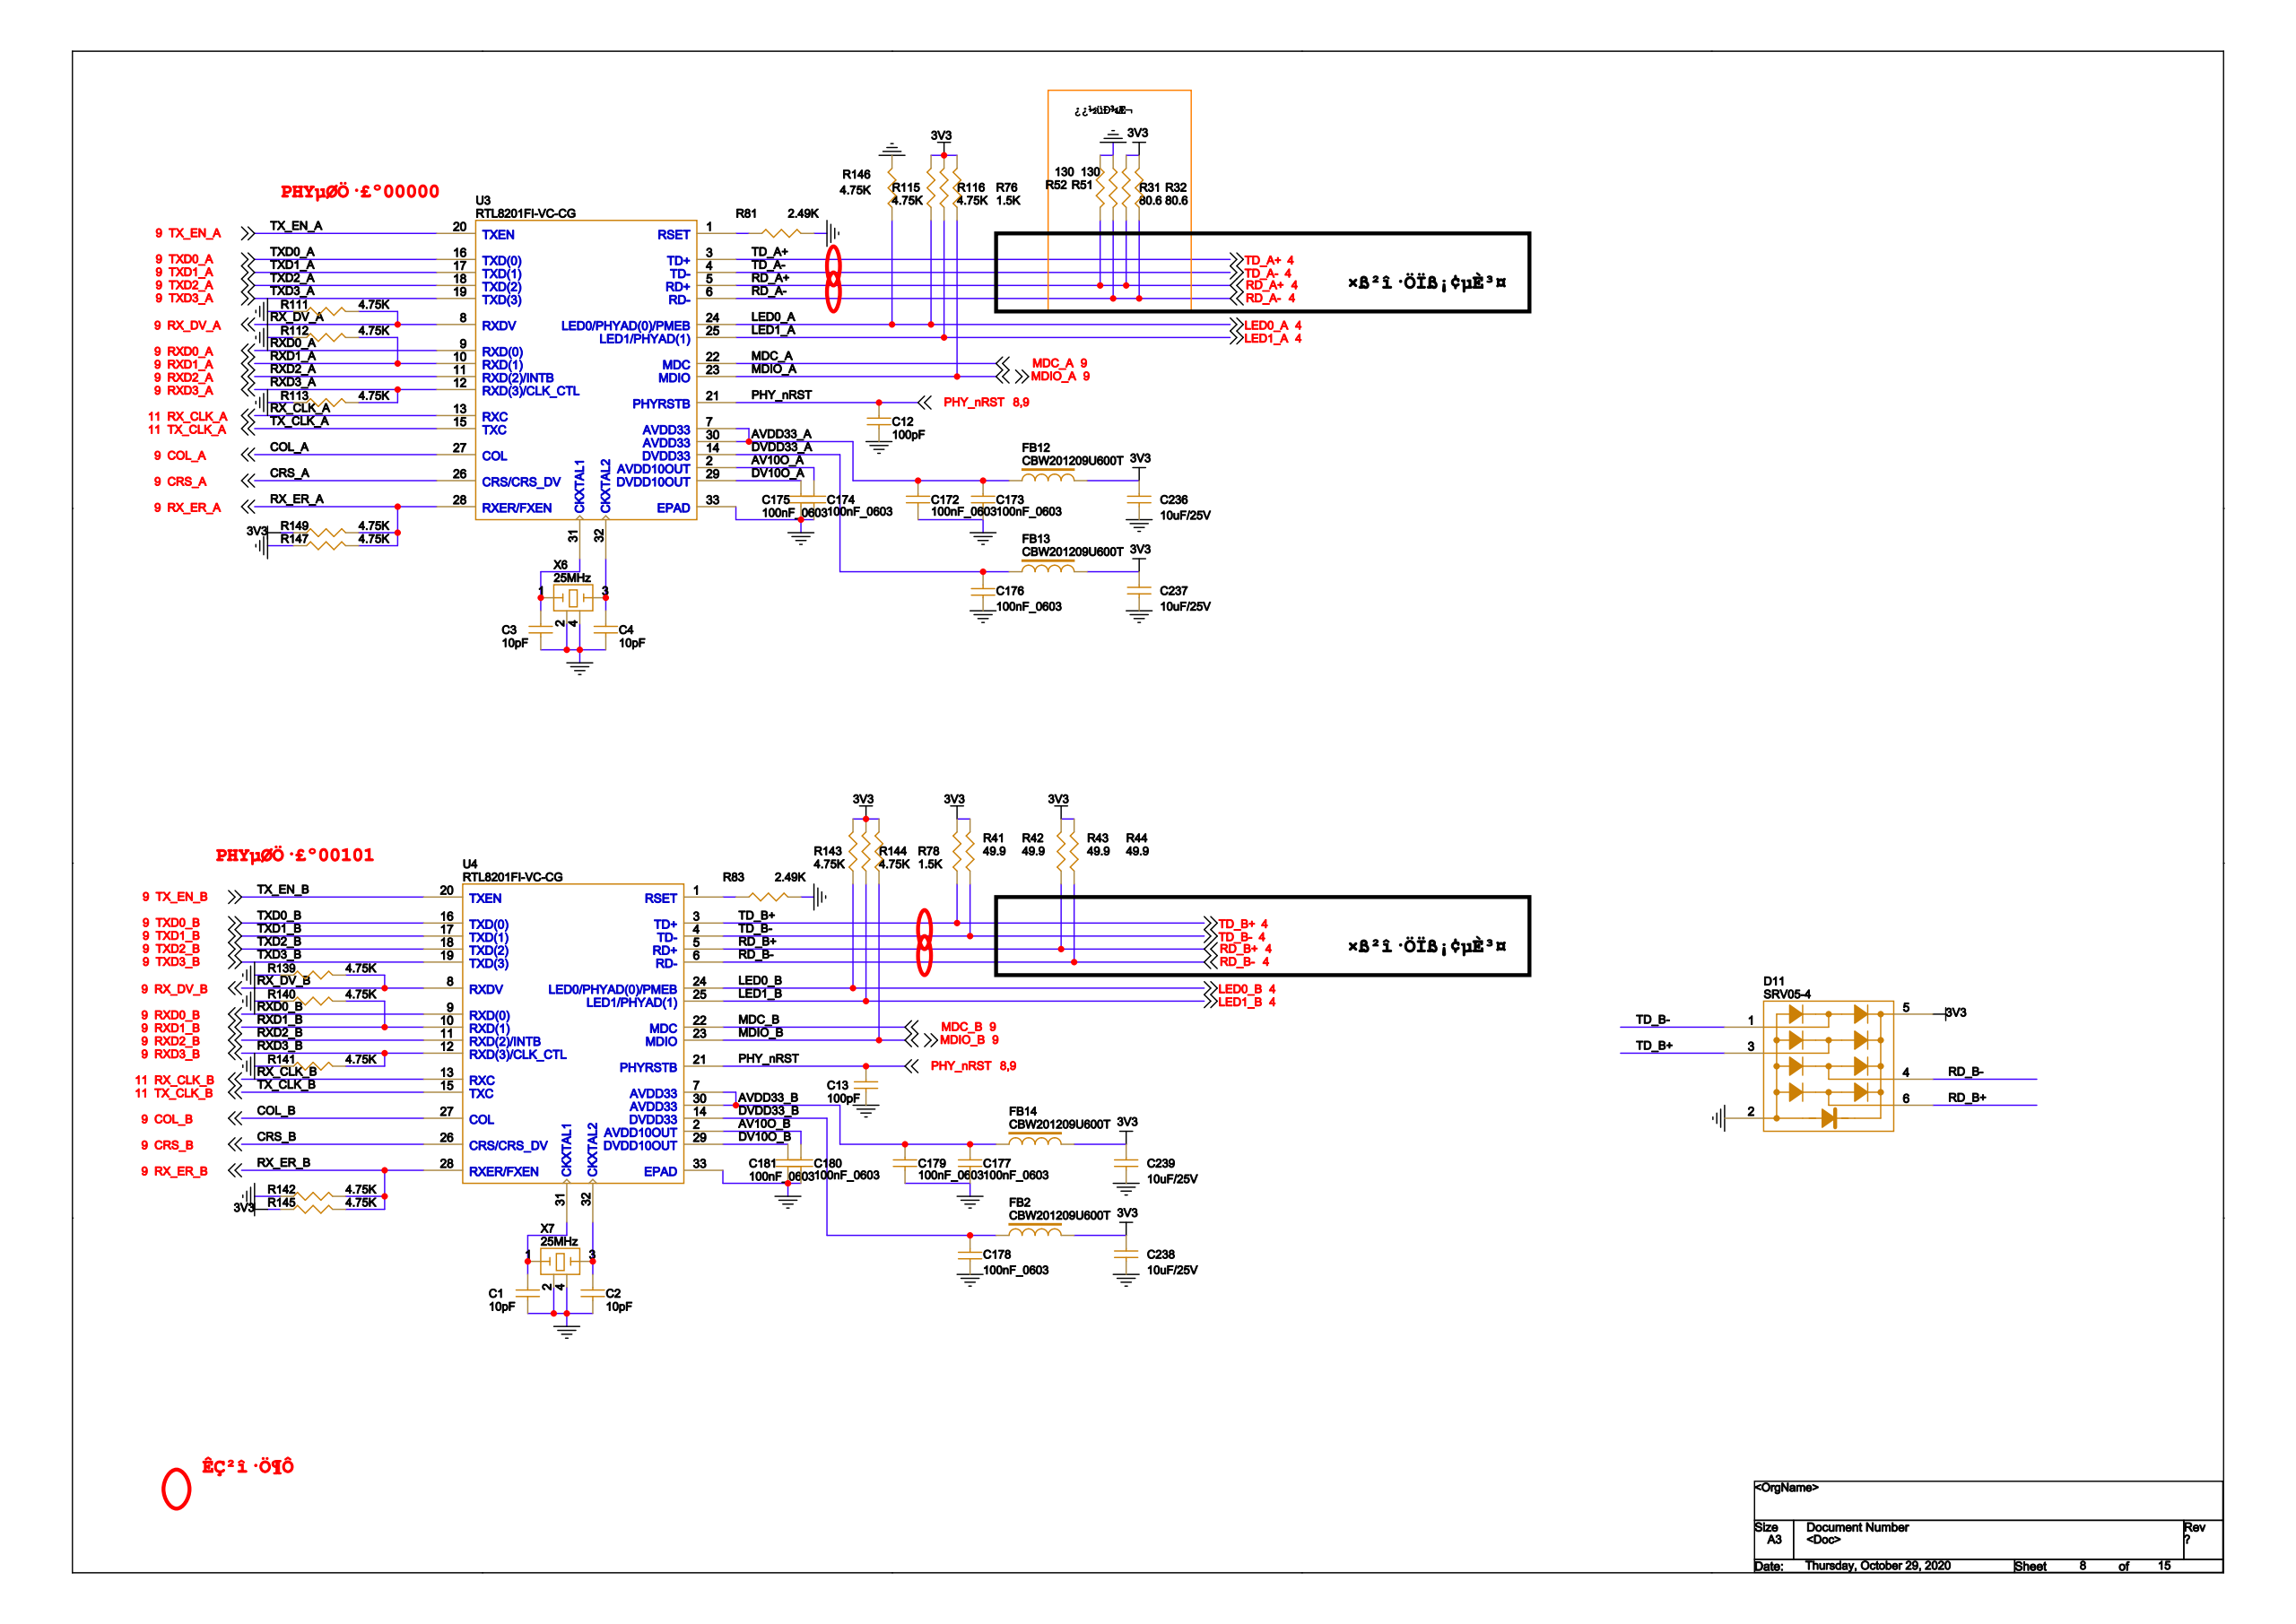Circuit board | Cadence Allegro | 406 parts | 392 nets | one sheet of the schematic
Parts on this sheet (reference | value | footprint):
C1 | 10pF | C_0603
C2 | 10pF | C_0603
C3 | 10pF | C_0603
C4 | 10pF | C_0603
C13 | 100pF | C_0603
C172 | 100nF_0603 | C_0603_104
C173 | 100nF_0603 | C_0603_104
C174 | 100nF_0603 | C_0603_104
C175 | 100nF_0603 | C_0603_104
C176 | 100nF_0603 | C_0603_104
C177 | 100nF_0603 | C_0603_104
C178 | 100nF_0603 | C_0603_104
C179 | 100nF_0603 | C_0603_104
C180 | 100nF_0603 | C_0603_104
C181 | 100nF_0603 | C_0603_104
C236 | 10uF/25V | C_0805_106
C237 | 10uF/25V | C_0805_106
C238 | 10uF/25V | C_0805_106
C239 | 10uF/25V | C_0805_106
D11 | SRV05-4 | D_SOT23_6
FB2 | CBW201209U600T | L_0805
FB12 | CBW201209U600T | L_0805
FB13 | CBW201209U600T | L_0805
FB14 | CBW201209U600T | L_0805
R31 | 80.6 | R_0603
R32 | 80.6 | R_0603
R41 | 49.9 | R_0603
R42 | 49.9 | R_0603
R43 | 49.9 | R_0603
R44 | 49.9 | R_0603
R51 | 130 | R_0603
R52 | 130 | R_0603
R76 | 1.5K | R_0603
R78 | 1.5K | R_0603
R81 | 2.49K | R_0603
R83 | 2.49K | R_0603
R111 | 4.75K | R_0603
R112 | 4.75K | R_0603
R113 | 4.75K | R_0603
R115 | 4.75K | R_0603
R116 | 4.75K | R_0603
R139 | 4.75K | R_0603
R140 | 4.75K | R_0603
R141 | 4.75K | R_0603
R142 | 4.75K | R_0603
R143 | 4.75K | R_0603
R144 | 4.75K | R_0603
R145 | 4.75K | R_0603
R146 | 4.75K | R_0603
R147 | 4.75K | R_0603
R149 | 4.75K | R_0603
U3 | RTL8201FI-VC-CG | U_QFN32_0_5
U4 | RTL8201FI-VC-CG | U_QFN32_0_5
X6 | 25MHz | XTAL3225
X7 | 25MHz | XTAL3225
Nets of these parts (net: part-pin ...):
GND: C1-2 C2-2 C3-2 C4-2 C13-2 C172-2 C173-2 C174-2 C175-2 C176-1 C177-2 C178-1 C179-2 C180-2 C181-2 C236-2 C237-2 C238-2 C239-2 D11-2 R51-1 R52-1 R81-1 R83-1 R111-1 R112-1 R113-1 R139-1 R140-1 R141-1 R142-1 R146-1 R147-1 X6-2 X6-4 X7-2 X7-4 U3-33 U4-33
TD_A+: U3-3
TD_A-: U3-4
RD_A+: R31-1 R52-2 U3-5
RD_A-: R32-1 R51-2 U3-6
TD_B+: D11-3 R41-1 U4-3
TD_B-: D11-1 R42-1 U4-4
LED0_A: R115-1 R146-2 U3-24
LED1_A: R116-1 U3-25
RD_B+: D11-6 R43-1 U4-5
RD_B-: D11-4 R44-1 U4-6
LED0_B: R143-1 U4-24
LED1_B: R144-1 U4-25
N20022459: C1-1 X7-1 U4-31
N20022457: C2-1 X7-3 U4-32
N20022567: C3-1 X6-1 U3-31
N20022565: C4-1 X6-3 U3-32
3V3: C236-1 C237-1 C238-1 C239-1 D11-5 FB2-1 FB12-1 FB13-1 FB14-1 R31-2 R32-2 R41-2 R42-2 R43-2 R44-2 R76-2 R78-2 R115-2 R116-2 R143-2 R144-2 R145-1 R149-1
PHY_NRST: C13-1 U3-21 U4-21
AVDD33_A: C172-1 C173-1 FB12-2 U3-7 U3-30
AV10O_A: C174-1 U3-2
DV10O_A: C175-1 U3-29
DVDD33_A: C176-2 FB13-2 U3-14
AVDD33_B: C177-1 C179-1 FB14-2 U4-7 U4-30
DVDD33_B: C178-2 FB2-2 U4-14
AV10O_B: C180-1 U4-2
DV10O_B: C181-1 U4-29
RX_DV_A: R111-2 U3-8
RXD1_A: R112-2 U3-10
RXD3_A: R113-2 U3-12
RX_DV_B: R139-2 U4-8
RXD1_B: R140-2 U4-10
RXD3_B: R141-2 U4-12
RX_ER_B: R142-2 R145-2 U4-28
RX_ER_A: R147-2 R149-2 U3-28
MDIO_A: R76-1 U3-23
MDIO_B: R78-1 U4-23
N20021756: R81-2 U3-1
N20022604: R83-2 U4-1
COL_A: U3-27
CRS_A: U3-26
MDC_A: U3-22
RX_CLK_A: U3-13
RXD0_A: U3-9
RXD2_A: U3-11
TX_CLK_A: U3-15
TXD0_A: U3-16
TXD1_A: U3-17
TXD2_A: U3-18
TXD3_A: U3-19
TX_EN_A: U3-20
COL_B: U4-27
CRS_B: U4-26
MDC_B: U4-22
RX_CLK_B: U4-13
RXD0_B: U4-9
RXD2_B: U4-11
TX_CLK_B: U4-15
TXD0_B: U4-16
TXD1_B: U4-17
TXD2_B: U4-18
TXD3_B: U4-19
TX_EN_B: U4-20